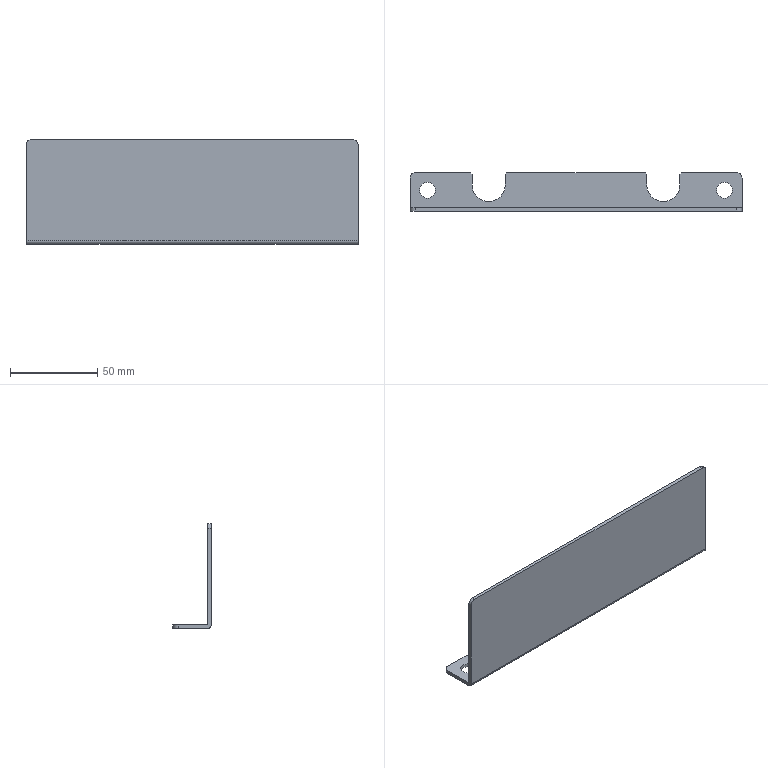Part | STEP file | gslz 2016.10.28-6_id946_x_t | 1 solid | 27 faces | box 190 x 22 x 60 mm | volume 28864 mm3 | plane 18 | cylinder 9 | commonest cylinder face diameters 6 x4 9 x2 19 x2 4 x1
STEP:
#1=CARTESIAN_POINT('',(59.5,282.,2.));
#2=VERTEX_POINT('',#1);
#3=CARTESIAN_POINT('',(59.5,288.,2.));
#4=VERTEX_POINT('',#3);
#5=CARTESIAN_POINT('',(59.5,280.75,2.));
#6=DIRECTION('',(0.,1.,0.));
#7=VECTOR('',#6,1.);
#8=LINE('',#5,#7);
#9=EDGE_CURVE('',#2,#4,#8,.T.);
#10=ORIENTED_EDGE('',*,*,#9,.T.);
#11=CARTESIAN_POINT('',(59.5,288.,0.));
#12=VERTEX_POINT('',#11);
#13=CARTESIAN_POINT('',(59.5,288.,0.));
#14=DIRECTION('',(0.,0.,-1.));
#15=VECTOR('',#14,1.);
#16=LINE('',#13,#15);
#17=EDGE_CURVE('',#4,#12,#16,.T.);
#18=ORIENTED_EDGE('',*,*,#17,.T.);
#19=CARTESIAN_POINT('',(59.5,282.,0.));
#20=VERTEX_POINT('',#19);
#21=CARTESIAN_POINT('',(59.5,280.75,0.));
#22=DIRECTION('',(0.,-1.,0.));
#23=VECTOR('',#22,1.);
#24=LINE('',#21,#23);
#25=EDGE_CURVE('',#12,#20,#24,.T.);
#26=ORIENTED_EDGE('',*,*,#25,.T.);
#27=CARTESIAN_POINT('',(59.5,282.,90.));
#28=DIRECTION('',(0.,0.,-1.));
#29=VECTOR('',#28,1.);
#30=LINE('',#27,#29);
#31=EDGE_CURVE('',#2,#20,#30,.T.);
#32=ORIENTED_EDGE('',*,*,#31,.F.);
#33=EDGE_LOOP('',(#10,#18,#26,#32));
#34=FACE_OUTER_BOUND('',#33,.T.);
#35=CARTESIAN_POINT('',(59.5,280.75,0.));
#36=DIRECTION('',(1.,0.,0.));
#37=DIRECTION('',(0.,0.,1.));
#38=AXIS2_PLACEMENT_3D('',#35,#36,#37);
#39=PLANE('',#38);
#40=ADVANCED_FACE('',(#34),#39,.F.);
#41=CARTESIAN_POINT('',(92.,289.,0.));
#42=VERTEX_POINT('',#41);
#43=CARTESIAN_POINT('',(60.5,289.,0.));
#44=VERTEX_POINT('',#43);
#45=CARTESIAN_POINT('',(0.000000002,289.,0.));
#46=DIRECTION('',(-1.,0.,0.));
#47=VECTOR('',#46,1.);
#48=LINE('',#45,#47);
#49=EDGE_CURVE('',#42,#44,#48,.T.);
#50=ORIENTED_EDGE('',*,*,#49,.T.);
#51=CARTESIAN_POINT('',(60.5,289.,2.));
#52=VERTEX_POINT('',#51);
#53=CARTESIAN_POINT('',(60.5,289.,2.));
#54=DIRECTION('',(0.,0.,1.));
#55=VECTOR('',#54,1.);
#56=LINE('',#53,#55);
#57=EDGE_CURVE('',#44,#52,#56,.T.);
#58=ORIENTED_EDGE('',*,*,#57,.T.);
#59=CARTESIAN_POINT('',(92.,289.,2.));
#60=VERTEX_POINT('',#59);
#61=CARTESIAN_POINT('',(96.45,289.,2.));
#62=DIRECTION('',(-1.,0.,0.));
#63=VECTOR('',#62,1.);
#64=LINE('',#61,#63);
#65=EDGE_CURVE('',#60,#52,#64,.T.);
#66=ORIENTED_EDGE('',*,*,#65,.F.);
#67=CARTESIAN_POINT('',(92.,289.,-221.492));
#68=DIRECTION('',(0.,0.,-1.));
#69=VECTOR('',#68,1.);
#70=LINE('',#67,#69);
#71=EDGE_CURVE('',#60,#42,#70,.T.);
#72=ORIENTED_EDGE('',*,*,#71,.T.);
#73=EDGE_LOOP('',(#50,#58,#66,#72));
#74=FACE_OUTER_BOUND('',#73,.T.);
#75=CARTESIAN_POINT('',(0.000000002,289.,-221.492));
#76=DIRECTION('',(0.,1.,0.));
#77=DIRECTION('',(0.,0.,1.));
#78=AXIS2_PLACEMENT_3D('',#75,#76,#77);
#79=PLANE('',#78);
#80=ADVANCED_FACE('',(#74),#79,.T.);
#81=ORIENTED_EDGE('',*,*,#65,.T.);
#82=CARTESIAN_POINT('',(67.475,295.975,2.));
#83=DIRECTION('',(-0.7071,-0.7071,0.));
#84=VECTOR('',#83,1.);
#85=LINE('',#82,#84);
#86=EDGE_CURVE('',#52,#4,#85,.T.);
#87=ORIENTED_EDGE('',*,*,#86,.T.);
#88=ORIENTED_EDGE('',*,*,#9,.F.);
#89=CARTESIAN_POINT('',(40.5,282.,2.));
#90=VERTEX_POINT('',#89);
#91=CARTESIAN_POINT('',(50.,282.,2.));
#92=DIRECTION('',(0.,0.,1.));
#93=DIRECTION('',(0.,-1.,0.));
#94=AXIS2_PLACEMENT_3D('',#91,#92,#93);
#95=CIRCLE('',#94,9.5);
#96=EDGE_CURVE('',#90,#2,#95,.T.);
#97=ORIENTED_EDGE('',*,*,#96,.F.);
#98=CARTESIAN_POINT('',(40.5,288.,2.));
#99=VERTEX_POINT('',#98);
#100=CARTESIAN_POINT('',(40.5,280.75,2.));
#101=DIRECTION('',(0.,-1.,0.));
#102=VECTOR('',#101,1.);
#103=LINE('',#100,#102);
#104=EDGE_CURVE('',#99,#90,#103,.T.);
#105=ORIENTED_EDGE('',*,*,#104,.F.);
#106=CARTESIAN_POINT('',(39.5,289.,2.));
#107=VERTEX_POINT('',#106);
#108=CARTESIAN_POINT('',(78.975,249.525,2.));
#109=DIRECTION('',(-0.7071,0.7071,0.));
#110=VECTOR('',#109,1.);
#111=LINE('',#108,#110);
#112=EDGE_CURVE('',#99,#107,#111,.T.);
#113=ORIENTED_EDGE('',*,*,#112,.T.);
#114=CARTESIAN_POINT('',(-39.5,289.,2.));
#115=VERTEX_POINT('',#114);
#116=CARTESIAN_POINT('',(96.45,289.,2.));
#117=DIRECTION('',(-1.,0.,0.));
#118=VECTOR('',#117,1.);
#119=LINE('',#116,#118);
#120=EDGE_CURVE('',#107,#115,#119,.T.);
#121=ORIENTED_EDGE('',*,*,#120,.T.);
#122=CARTESIAN_POINT('',(-40.5,288.,2.));
#123=VERTEX_POINT('',#122);
#124=CARTESIAN_POINT('',(17.475,345.975,2.));
#125=DIRECTION('',(-0.7071,-0.7071,0.));
#126=VECTOR('',#125,1.);
#127=LINE('',#124,#126);
#128=EDGE_CURVE('',#115,#123,#127,.T.);
#129=ORIENTED_EDGE('',*,*,#128,.T.);
#130=CARTESIAN_POINT('',(-40.5,282.,2.));
#131=VERTEX_POINT('',#130);
#132=CARTESIAN_POINT('',(-40.5,280.75,2.));
#133=DIRECTION('',(0.,1.,0.));
#134=VECTOR('',#133,1.);
#135=LINE('',#132,#134);
#136=EDGE_CURVE('',#131,#123,#135,.T.);
#137=ORIENTED_EDGE('',*,*,#136,.F.);
#138=CARTESIAN_POINT('',(-59.5,282.,2.));
#139=VERTEX_POINT('',#138);
#140=CARTESIAN_POINT('',(-50.,282.,2.));
#141=DIRECTION('',(0.,0.,1.));
#142=DIRECTION('',(0.,-1.,0.));
#143=AXIS2_PLACEMENT_3D('',#140,#141,#142);
#144=CIRCLE('',#143,9.5);
#145=EDGE_CURVE('',#139,#131,#144,.T.);
#146=ORIENTED_EDGE('',*,*,#145,.F.);
#147=CARTESIAN_POINT('',(-59.5,288.,2.));
#148=VERTEX_POINT('',#147);
#149=CARTESIAN_POINT('',(-59.5,280.75,2.));
#150=DIRECTION('',(0.,-1.,0.));
#151=VECTOR('',#150,1.);
#152=LINE('',#149,#151);
#153=EDGE_CURVE('',#148,#139,#152,.T.);
#154=ORIENTED_EDGE('',*,*,#153,.F.);
#155=CARTESIAN_POINT('',(-60.5,289.,2.));
#156=VERTEX_POINT('',#155);
#157=CARTESIAN_POINT('',(28.975,199.525,2.));
#158=DIRECTION('',(-0.7071,0.7071,0.));
#159=VECTOR('',#158,1.);
#160=LINE('',#157,#159);
#161=EDGE_CURVE('',#148,#156,#160,.T.);
#162=ORIENTED_EDGE('',*,*,#161,.T.);
#163=CARTESIAN_POINT('',(-92.,289.,2.));
#164=VERTEX_POINT('',#163);
#165=CARTESIAN_POINT('',(96.45,289.,2.));
#166=DIRECTION('',(-1.,0.,0.));
#167=VECTOR('',#166,1.);
#168=LINE('',#165,#167);
#169=EDGE_CURVE('',#156,#164,#168,.T.);
#170=ORIENTED_EDGE('',*,*,#169,.T.);
#171=CARTESIAN_POINT('',(-95.,286.,2.));
#172=VERTEX_POINT('',#171);
#173=CARTESIAN_POINT('',(-92.,286.,2.));
#174=DIRECTION('',(0.,0.,1.));
#175=DIRECTION('',(0.,-1.,0.));
#176=AXIS2_PLACEMENT_3D('',#173,#174,#175);
#177=CIRCLE('',#176,3.);
#178=EDGE_CURVE('',#164,#172,#177,.T.);
#179=ORIENTED_EDGE('',*,*,#178,.T.);
#180=CARTESIAN_POINT('',(-95.,269.,2.));
#181=VERTEX_POINT('',#180);
#182=CARTESIAN_POINT('',(-95.,267.,2.));
#183=DIRECTION('',(0.,1.,0.));
#184=VECTOR('',#183,1.);
#185=LINE('',#182,#184);
#186=EDGE_CURVE('',#181,#172,#185,.T.);
#187=ORIENTED_EDGE('',*,*,#186,.F.);
#188=CARTESIAN_POINT('',(95.,269.,2.));
#189=VERTEX_POINT('',#188);
#190=CARTESIAN_POINT('',(-84.45,269.,2.));
#191=DIRECTION('',(-1.,0.,0.));
#192=VECTOR('',#191,1.);
#193=LINE('',#190,#192);
#194=EDGE_CURVE('',#189,#181,#193,.T.);
#195=ORIENTED_EDGE('',*,*,#194,.F.);
#196=CARTESIAN_POINT('',(95.,286.,2.));
#197=VERTEX_POINT('',#196);
#198=CARTESIAN_POINT('',(95.,267.,2.));
#199=DIRECTION('',(0.,-1.,0.));
#200=VECTOR('',#199,1.);
#201=LINE('',#198,#200);
#202=EDGE_CURVE('',#197,#189,#201,.T.);
#203=ORIENTED_EDGE('',*,*,#202,.F.);
#204=CARTESIAN_POINT('',(92.,286.,2.));
#205=DIRECTION('',(0.,0.,1.));
#206=DIRECTION('',(0.,-1.,0.));
#207=AXIS2_PLACEMENT_3D('',#204,#205,#206);
#208=CIRCLE('',#207,3.);
#209=EDGE_CURVE('',#197,#60,#208,.T.);
#210=ORIENTED_EDGE('',*,*,#209,.T.);
#211=EDGE_LOOP('',(#81,#87,#88,#97,#105,#113,#121,#129,#137,#146,#154,#162,#170,#179,#187,#195,#203,#210));
#212=FACE_BOUND('',#211,.T.);
#213=CARTESIAN_POINT('',(-89.5,279.,2.));
#214=VERTEX_POINT('',#213);
#215=CARTESIAN_POINT('',(-85.,279.,2.));
#216=DIRECTION('',(0.,0.,-1.));
#217=DIRECTION('',(-1.,0.,0.));
#218=AXIS2_PLACEMENT_3D('',#215,#216,#217);
#219=CIRCLE('',#218,4.5);
#220=EDGE_CURVE('',#214,#214,#219,.T.);
#221=ORIENTED_EDGE('',*,*,#220,.T.);
#222=EDGE_LOOP('',(#221));
#223=FACE_BOUND('',#222,.T.);
#224=CARTESIAN_POINT('',(80.5,279.,2.));
#225=VERTEX_POINT('',#224);
#226=CARTESIAN_POINT('',(85.,279.,2.));
#227=DIRECTION('',(0.,0.,-1.));
#228=DIRECTION('',(-1.,0.,0.));
#229=AXIS2_PLACEMENT_3D('',#226,#227,#228);
#230=CIRCLE('',#229,4.5);
#231=EDGE_CURVE('',#225,#225,#230,.T.);
#232=ORIENTED_EDGE('',*,*,#231,.T.);
#233=EDGE_LOOP('',(#232));
#234=FACE_BOUND('',#233,.T.);
#235=CARTESIAN_POINT('',(96.45,267.,2.));
#236=DIRECTION('',(0.,0.,1.));
#237=DIRECTION('',(-1.,0.,0.));
#238=AXIS2_PLACEMENT_3D('',#235,#236,#237);
#239=PLANE('',#238);
#240=ADVANCED_FACE('',(#212,#223,#234),#239,.T.);
#241=ORIENTED_EDGE('',*,*,#25,.F.);
#242=CARTESIAN_POINT('',(-41.75,186.75,0.));
#243=DIRECTION('',(0.7071,0.7071,0.));
#244=VECTOR('',#243,1.);
#245=LINE('',#242,#244);
#246=EDGE_CURVE('',#12,#44,#245,.T.);
#247=ORIENTED_EDGE('',*,*,#246,.T.);
#248=ORIENTED_EDGE('',*,*,#49,.F.);
#249=CARTESIAN_POINT('',(95.,286.,0.));
#250=VERTEX_POINT('',#249);
#251=CARTESIAN_POINT('',(92.,286.,0.));
#252=DIRECTION('',(0.,0.,-1.));
#253=DIRECTION('',(0.,-1.,0.));
#254=AXIS2_PLACEMENT_3D('',#251,#252,#253);
#255=CIRCLE('',#254,3.);
#256=EDGE_CURVE('',#42,#250,#255,.T.);
#257=ORIENTED_EDGE('',*,*,#256,.T.);
#258=CARTESIAN_POINT('',(95.,269.,0.));
#259=VERTEX_POINT('',#258);
#260=CARTESIAN_POINT('',(95.,155.,0.));
#261=DIRECTION('',(0.,1.,0.));
#262=VECTOR('',#261,1.);
#263=LINE('',#260,#262);
#264=EDGE_CURVE('',#259,#250,#263,.T.);
#265=ORIENTED_EDGE('',*,*,#264,.F.);
#266=CARTESIAN_POINT('',(-95.,269.,0.));
#267=VERTEX_POINT('',#266);
#268=CARTESIAN_POINT('',(-95.,269.,0.));
#269=DIRECTION('',(-1.,0.,0.));
#270=VECTOR('',#269,1.);
#271=LINE('',#268,#270);
#272=EDGE_CURVE('',#259,#267,#271,.T.);
#273=ORIENTED_EDGE('',*,*,#272,.T.);
#274=CARTESIAN_POINT('',(-95.,286.,0.));
#275=VERTEX_POINT('',#274);
#276=CARTESIAN_POINT('',(-95.,155.,0.));
#277=DIRECTION('',(0.,1.,0.));
#278=VECTOR('',#277,1.);
#279=LINE('',#276,#278);
#280=EDGE_CURVE('',#267,#275,#279,.T.);
#281=ORIENTED_EDGE('',*,*,#280,.T.);
#282=CARTESIAN_POINT('',(-92.,289.,0.));
#283=VERTEX_POINT('',#282);
#284=CARTESIAN_POINT('',(-92.,286.,0.));
#285=DIRECTION('',(0.,0.,-1.));
#286=DIRECTION('',(0.,-1.,0.));
#287=AXIS2_PLACEMENT_3D('',#284,#285,#286);
#288=CIRCLE('',#287,3.);
#289=EDGE_CURVE('',#275,#283,#288,.T.);
#290=ORIENTED_EDGE('',*,*,#289,.T.);
#291=CARTESIAN_POINT('',(-60.5,289.,0.));
#292=VERTEX_POINT('',#291);
#293=CARTESIAN_POINT('',(0.000000002,289.,0.));
#294=DIRECTION('',(-1.,0.,0.));
#295=VECTOR('',#294,1.);
#296=LINE('',#293,#295);
#297=EDGE_CURVE('',#292,#283,#296,.T.);
#298=ORIENTED_EDGE('',*,*,#297,.F.);
#299=CARTESIAN_POINT('',(-59.5,288.,0.));
#300=VERTEX_POINT('',#299);
#301=CARTESIAN_POINT('',(31.75,196.75,0.));
#302=DIRECTION('',(0.7071,-0.7071,0.));
#303=VECTOR('',#302,1.);
#304=LINE('',#301,#303);
#305=EDGE_CURVE('',#292,#300,#304,.T.);
#306=ORIENTED_EDGE('',*,*,#305,.T.);
#307=CARTESIAN_POINT('',(-59.5,282.,0.));
#308=VERTEX_POINT('',#307);
#309=CARTESIAN_POINT('',(-59.5,280.75,0.));
#310=DIRECTION('',(0.,-1.,0.));
#311=VECTOR('',#310,1.);
#312=LINE('',#309,#311);
#313=EDGE_CURVE('',#300,#308,#312,.T.);
#314=ORIENTED_EDGE('',*,*,#313,.T.);
#315=CARTESIAN_POINT('',(-40.5,282.,0.));
#316=VERTEX_POINT('',#315);
#317=CARTESIAN_POINT('',(-50.,282.,0.));
#318=DIRECTION('',(0.,0.,-1.));
#319=DIRECTION('',(-1.,0.,0.));
#320=AXIS2_PLACEMENT_3D('',#317,#318,#319);
#321=CIRCLE('',#320,9.5);
#322=EDGE_CURVE('',#316,#308,#321,.T.);
#323=ORIENTED_EDGE('',*,*,#322,.F.);
#324=CARTESIAN_POINT('',(-40.5,288.,0.));
#325=VERTEX_POINT('',#324);
#326=CARTESIAN_POINT('',(-40.5,280.75,0.));
#327=DIRECTION('',(0.,1.,0.));
#328=VECTOR('',#327,1.);
#329=LINE('',#326,#328);
#330=EDGE_CURVE('',#316,#325,#329,.T.);
#331=ORIENTED_EDGE('',*,*,#330,.T.);
#332=CARTESIAN_POINT('',(-39.5,289.,0.));
#333=VERTEX_POINT('',#332);
#334=CARTESIAN_POINT('',(-91.75,236.75,0.));
#335=DIRECTION('',(0.7071,0.7071,0.));
#336=VECTOR('',#335,1.);
#337=LINE('',#334,#336);
#338=EDGE_CURVE('',#325,#333,#337,.T.);
#339=ORIENTED_EDGE('',*,*,#338,.T.);
#340=CARTESIAN_POINT('',(39.5,289.,0.));
#341=VERTEX_POINT('',#340);
#342=CARTESIAN_POINT('',(0.000000002,289.,0.));
#343=DIRECTION('',(-1.,0.,0.));
#344=VECTOR('',#343,1.);
#345=LINE('',#342,#344);
#346=EDGE_CURVE('',#341,#333,#345,.T.);
#347=ORIENTED_EDGE('',*,*,#346,.F.);
#348=CARTESIAN_POINT('',(40.5,288.,0.));
#349=VERTEX_POINT('',#348);
#350=CARTESIAN_POINT('',(81.75,246.75,0.));
#351=DIRECTION('',(0.7071,-0.7071,0.));
#352=VECTOR('',#351,1.);
#353=LINE('',#350,#352);
#354=EDGE_CURVE('',#341,#349,#353,.T.);
#355=ORIENTED_EDGE('',*,*,#354,.T.);
#356=CARTESIAN_POINT('',(40.5,282.,0.));
#357=VERTEX_POINT('',#356);
#358=CARTESIAN_POINT('',(40.5,280.75,0.));
#359=DIRECTION('',(0.,-1.,0.));
#360=VECTOR('',#359,1.);
#361=LINE('',#358,#360);
#362=EDGE_CURVE('',#349,#357,#361,.T.);
#363=ORIENTED_EDGE('',*,*,#362,.T.);
#364=CARTESIAN_POINT('',(50.,282.,0.));
#365=DIRECTION('',(0.,0.,-1.));
#366=DIRECTION('',(-1.,0.,0.));
#367=AXIS2_PLACEMENT_3D('',#364,#365,#366);
#368=CIRCLE('',#367,9.5);
#369=EDGE_CURVE('',#20,#357,#368,.T.);
#370=ORIENTED_EDGE('',*,*,#369,.F.);
#371=EDGE_LOOP('',(#241,#247,#248,#257,#265,#273,#281,#290,#298,#306,#314,#323,#331,#339,#347,#355,#363,#370));
#372=FACE_BOUND('',#371,.T.);
#373=CARTESIAN_POINT('',(80.5,279.,0.));
#374=VERTEX_POINT('',#373);
#375=CARTESIAN_POINT('',(85.,279.,0.));
#376=DIRECTION('',(0.,0.,-1.));
#377=DIRECTION('',(-1.,0.,0.));
#378=AXIS2_PLACEMENT_3D('',#375,#376,#377);
#379=CIRCLE('',#378,4.5);
#380=EDGE_CURVE('',#374,#374,#379,.T.);
#381=ORIENTED_EDGE('',*,*,#380,.F.);
#382=EDGE_LOOP('',(#381));
#383=FACE_BOUND('',#382,.T.);
#384=CARTESIAN_POINT('',(-89.5,279.,0.));
#385=VERTEX_POINT('',#384);
#386=CARTESIAN_POINT('',(-85.,279.,0.));
#387=DIRECTION('',(0.,0.,-1.));
#388=DIRECTION('',(-1.,0.,0.));
#389=AXIS2_PLACEMENT_3D('',#386,#387,#388);
#390=CIRCLE('',#389,4.5);
#391=EDGE_CURVE('',#385,#385,#390,.T.);
#392=ORIENTED_EDGE('',*,*,#391,.F.);
#393=EDGE_LOOP('',(#392));
#394=FACE_BOUND('',#393,.T.);
#395=CARTESIAN_POINT('',(-10.,155.,0.));
#396=DIRECTION('',(0.,0.,1.));
#397=DIRECTION('',(-1.,0.,0.));
#398=AXIS2_PLACEMENT_3D('',#395,#396,#397);
#399=PLANE('',#398);
#400=ADVANCED_FACE('',(#372,#383,#394),#399,.F.);
#401=ORIENTED_EDGE('',*,*,#120,.F.);
#402=CARTESIAN_POINT('',(39.5,289.,0.));
#403=DIRECTION('',(0.,0.,-1.));
#404=VECTOR('',#403,1.);
#405=LINE('',#402,#404);
#406=EDGE_CURVE('',#107,#341,#405,.T.);
#407=ORIENTED_EDGE('',*,*,#406,.T.);
#408=ORIENTED_EDGE('',*,*,#346,.T.);
#409=CARTESIAN_POINT('',(-39.5,289.,2.));
#410=DIRECTION('',(0.,0.,1.));
#411=VECTOR('',#410,1.);
#412=LINE('',#409,#411);
#413=EDGE_CURVE('',#333,#115,#412,.T.);
#414=ORIENTED_EDGE('',*,*,#413,.T.);
#415=EDGE_LOOP('',(#401,#407,#408,#414));
#416=FACE_OUTER_BOUND('',#415,.T.);
#417=CARTESIAN_POINT('',(0.000000002,289.,-221.492));
#418=DIRECTION('',(0.,1.,0.));
#419=DIRECTION('',(0.,0.,1.));
#420=AXIS2_PLACEMENT_3D('',#417,#418,#419);
#421=PLANE('',#420);
#422=ADVANCED_FACE('',(#416),#421,.T.);
#423=ORIENTED_EDGE('',*,*,#186,.T.);
#424=CARTESIAN_POINT('',(-95.,286.,0.));
#425=DIRECTION('',(0.,0.,-1.));
#426=VECTOR('',#425,1.);
#427=LINE('',#424,#426);
#428=EDGE_CURVE('',#172,#275,#427,.T.);
#429=ORIENTED_EDGE('',*,*,#428,.T.);
#430=ORIENTED_EDGE('',*,*,#280,.F.);
#431=CARTESIAN_POINT('',(-95.,267.,2.));
#432=VERTEX_POINT('',#431);
#433=CARTESIAN_POINT('',(-95.,269.,2.));
#434=DIRECTION('',(-1.,0.,0.));
#435=DIRECTION('',(0.,0.,1.));
#436=AXIS2_PLACEMENT_3D('',#433,#434,#435);
#437=CIRCLE('',#436,2.);
#438=EDGE_CURVE('',#267,#432,#437,.T.);
#439=ORIENTED_EDGE('',*,*,#438,.T.);
#440=CARTESIAN_POINT('',(-95.,267.,57.));
#441=VERTEX_POINT('',#440);
#442=CARTESIAN_POINT('',(-95.,267.,2.));
#443=DIRECTION('',(0.,0.,-1.));
#444=VECTOR('',#443,1.);
#445=LINE('',#442,#444);
#446=EDGE_CURVE('',#441,#432,#445,.T.);
#447=ORIENTED_EDGE('',*,*,#446,.F.);
#448=CARTESIAN_POINT('',(-95.,269.,57.));
#449=VERTEX_POINT('',#448);
#450=CARTESIAN_POINT('',(-95.,0.,57.));
#451=DIRECTION('',(0.,1.,0.));
#452=VECTOR('',#451,1.);
#453=LINE('',#450,#452);
#454=EDGE_CURVE('',#441,#449,#453,.T.);
#455=ORIENTED_EDGE('',*,*,#454,.T.);
#456=CARTESIAN_POINT('',(-95.,269.,2.));
#457=DIRECTION('',(0.,0.,-1.));
#458=VECTOR('',#457,1.);
#459=LINE('',#456,#458);
#460=EDGE_CURVE('',#449,#181,#459,.T.);
#461=ORIENTED_EDGE('',*,*,#460,.T.);
#462=EDGE_LOOP('',(#423,#429,#430,#439,#447,#455,#461));
#463=FACE_OUTER_BOUND('',#462,.T.);
#464=CARTESIAN_POINT('',(-95.,0.,0.));
#465=DIRECTION('',(-1.,0.,0.));
#466=DIRECTION('',(0.,0.,-1.));
#467=AXIS2_PLACEMENT_3D('',#464,#465,#466);
#468=PLANE('',#467);
#469=ADVANCED_FACE('',(#463),#468,.T.);
#470=ORIENTED_EDGE('',*,*,#264,.T.);
#471=CARTESIAN_POINT('',(95.,286.,0.));
#472=DIRECTION('',(0.,0.,1.));
#473=VECTOR('',#472,1.);
#474=LINE('',#471,#473);
#475=EDGE_CURVE('',#250,#197,#474,.T.);
#476=ORIENTED_EDGE('',*,*,#475,.T.);
#477=ORIENTED_EDGE('',*,*,#202,.T.);
#478=CARTESIAN_POINT('',(95.,269.,57.));
#479=VERTEX_POINT('',#478);
#480=CARTESIAN_POINT('',(95.,269.,2.));
#481=DIRECTION('',(0.,0.,1.));
#482=VECTOR('',#481,1.);
#483=LINE('',#480,#482);
#484=EDGE_CURVE('',#189,#479,#483,.T.);
#485=ORIENTED_EDGE('',*,*,#484,.T.);
#486=CARTESIAN_POINT('',(95.,267.,57.));
#487=VERTEX_POINT('',#486);
#488=CARTESIAN_POINT('',(95.,0.,57.));
#489=DIRECTION('',(0.,-1.,0.));
#490=VECTOR('',#489,1.);
#491=LINE('',#488,#490);
#492=EDGE_CURVE('',#479,#487,#491,.T.);
#493=ORIENTED_EDGE('',*,*,#492,.T.);
#494=CARTESIAN_POINT('',(95.,267.,2.));
#495=VERTEX_POINT('',#494);
#496=CARTESIAN_POINT('',(95.,267.,2.));
#497=DIRECTION('',(0.,0.,1.));
#498=VECTOR('',#497,1.);
#499=LINE('',#496,#498);
#500=EDGE_CURVE('',#495,#487,#499,.T.);
#501=ORIENTED_EDGE('',*,*,#500,.F.);
#502=CARTESIAN_POINT('',(95.,269.,2.));
#503=DIRECTION('',(1.,0.,0.));
#504=DIRECTION('',(0.,0.,-1.));
#505=AXIS2_PLACEMENT_3D('',#502,#503,#504);
#506=CIRCLE('',#505,2.);
#507=EDGE_CURVE('',#495,#259,#506,.T.);
#508=ORIENTED_EDGE('',*,*,#507,.T.);
#509=EDGE_LOOP('',(#470,#476,#477,#485,#493,#501,#508));
#510=FACE_OUTER_BOUND('',#509,.T.);
#511=CARTESIAN_POINT('',(95.,0.,0.));
#512=DIRECTION('',(1.,0.,0.));
#513=DIRECTION('',(0.,0.,1.));
#514=AXIS2_PLACEMENT_3D('',#511,#512,#513);
#515=PLANE('',#514);
#516=ADVANCED_FACE('',(#510),#515,.T.);
#517=CARTESIAN_POINT('',(-92.,269.,60.));
#518=VERTEX_POINT('',#517);
#519=CARTESIAN_POINT('',(92.,269.,60.));
#520=VERTEX_POINT('',#519);
#521=CARTESIAN_POINT('',(-89.5,269.,60.));
#522=DIRECTION('',(1.,0.,0.));
#523=VECTOR('',#522,1.);
#524=LINE('',#521,#523);
#525=EDGE_CURVE('',#518,#520,#524,.T.);
#526=ORIENTED_EDGE('',*,*,#525,.F.);
#527=CARTESIAN_POINT('',(-92.,267.,60.));
#528=VERTEX_POINT('',#527);
#529=CARTESIAN_POINT('',(-92.,200.,60.));
#530=DIRECTION('',(0.,-1.,0.));
#531=VECTOR('',#530,1.);
#532=LINE('',#529,#531);
#533=EDGE_CURVE('',#518,#528,#532,.T.);
#534=ORIENTED_EDGE('',*,*,#533,.T.);
#535=CARTESIAN_POINT('',(92.,267.,60.));
#536=VERTEX_POINT('',#535);
#537=CARTESIAN_POINT('',(-89.5,267.,60.));
#538=DIRECTION('',(1.,0.,0.));
#539=VECTOR('',#538,1.);
#540=LINE('',#537,#539);
#541=EDGE_CURVE('',#528,#536,#540,.T.);
#542=ORIENTED_EDGE('',*,*,#541,.T.);
#543=CARTESIAN_POINT('',(92.,200.,60.));
#544=DIRECTION('',(0.,1.,0.));
#545=VECTOR('',#544,1.);
#546=LINE('',#543,#545);
#547=EDGE_CURVE('',#536,#520,#546,.T.);
#548=ORIENTED_EDGE('',*,*,#547,.T.);
#549=EDGE_LOOP('',(#526,#534,#542,#548));
#550=FACE_OUTER_BOUND('',#549,.T.);
#551=CARTESIAN_POINT('',(-89.5,200.,60.));
#552=DIRECTION('',(0.,0.,1.));
#553=DIRECTION('',(-1.,0.,0.));
#554=AXIS2_PLACEMENT_3D('',#551,#552,#553);
#555=PLANE('',#554);
#556=ADVANCED_FACE('',(#550),#555,.T.);
#557=ORIENTED_EDGE('',*,*,#169,.F.);
#558=CARTESIAN_POINT('',(-60.5,289.,0.));
#559=DIRECTION('',(0.,0.,-1.));
#560=VECTOR('',#559,1.);
#561=LINE('',#558,#560);
#562=EDGE_CURVE('',#156,#292,#561,.T.);
#563=ORIENTED_EDGE('',*,*,#562,.T.);
#564=ORIENTED_EDGE('',*,*,#297,.T.);
#565=CARTESIAN_POINT('',(-92.,289.,-221.492));
#566=DIRECTION('',(0.,0.,1.));
#567=VECTOR('',#566,1.);
#568=LINE('',#565,#567);
#569=EDGE_CURVE('',#283,#164,#568,.T.);
#570=ORIENTED_EDGE('',*,*,#569,.T.);
#571=EDGE_LOOP('',(#557,#563,#564,#570));
#572=FACE_OUTER_BOUND('',#571,.T.);
#573=CARTESIAN_POINT('',(0.000000002,289.,-221.492));
#574=DIRECTION('',(0.,1.,0.));
#575=DIRECTION('',(0.,0.,1.));
#576=AXIS2_PLACEMENT_3D('',#573,#574,#575);
#577=PLANE('',#576);
#578=ADVANCED_FACE('',(#572),#577,.T.);
#579=ORIENTED_EDGE('',*,*,#541,.F.);
#580=CARTESIAN_POINT('',(-92.,267.,57.));
#581=DIRECTION('',(0.,-1.,0.));
#582=DIRECTION('',(-1.,0.,0.));
#583=AXIS2_PLACEMENT_3D('',#580,#581,#582);
#584=CIRCLE('',#583,3.);
#585=EDGE_CURVE('',#528,#441,#584,.T.);
#586=ORIENTED_EDGE('',*,*,#585,.T.);
#587=ORIENTED_EDGE('',*,*,#446,.T.);
#588=CARTESIAN_POINT('',(95.,267.,2.));
#589=DIRECTION('',(1.,0.,0.));
#590=VECTOR('',#589,1.);
#591=LINE('',#588,#590);
#592=EDGE_CURVE('',#432,#495,#591,.T.);
#593=ORIENTED_EDGE('',*,*,#592,.T.);
#594=ORIENTED_EDGE('',*,*,#500,.T.);
#595=CARTESIAN_POINT('',(92.,267.,57.));
#596=DIRECTION('',(0.,-1.,0.));
#597=DIRECTION('',(-1.,0.,0.));
#598=AXIS2_PLACEMENT_3D('',#595,#596,#597);
#599=CIRCLE('',#598,3.);
#600=EDGE_CURVE('',#487,#536,#599,.T.);
#601=ORIENTED_EDGE('',*,*,#600,.T.);
#602=EDGE_LOOP('',(#579,#586,#587,#593,#594,#601));
#603=FACE_OUTER_BOUND('',#602,.T.);
#604=CARTESIAN_POINT('',(-89.45,267.,2.));
#605=DIRECTION('',(0.,1.,0.));
#606=DIRECTION('',(0.,0.,1.));
#607=AXIS2_PLACEMENT_3D('',#604,#605,#606);
#608=PLANE('',#607);
#609=ADVANCED_FACE('',(#603),#608,.F.);
#610=ORIENTED_EDGE('',*,*,#460,.F.);
#611=CARTESIAN_POINT('',(-92.,269.,57.));
#612=DIRECTION('',(0.,1.,0.));
#613=DIRECTION('',(-1.,0.,0.));
#614=AXIS2_PLACEMENT_3D('',#611,#612,#613);
#615=CIRCLE('',#614,3.);
#616=EDGE_CURVE('',#449,#518,#615,.T.);
#617=ORIENTED_EDGE('',*,*,#616,.T.);
#618=ORIENTED_EDGE('',*,*,#525,.T.);
#619=CARTESIAN_POINT('',(92.,269.,57.));
#620=DIRECTION('',(0.,1.,0.));
#621=DIRECTION('',(-1.,0.,0.));
#622=AXIS2_PLACEMENT_3D('',#619,#620,#621);
#623=CIRCLE('',#622,3.);
#624=EDGE_CURVE('',#520,#479,#623,.T.);
#625=ORIENTED_EDGE('',*,*,#624,.T.);
#626=ORIENTED_EDGE('',*,*,#484,.F.);
#627=ORIENTED_EDGE('',*,*,#194,.T.);
#628=EDGE_LOOP('',(#610,#617,#618,#625,#626,#627));
#629=FACE_OUTER_BOUND('',#628,.T.);
#630=CARTESIAN_POINT('',(-89.45,269.,2.));
#631=DIRECTION('',(0.,1.,0.));
#632=DIRECTION('',(0.,0.,1.));
#633=AXIS2_PLACEMENT_3D('',#630,#631,#632);
#634=PLANE('',#633);
#635=ADVANCED_FACE('',(#629),#634,.T.);
#636=ORIENTED_EDGE('',*,*,#438,.F.);
#637=ORIENTED_EDGE('',*,*,#272,.F.);
#638=ORIENTED_EDGE('',*,*,#507,.F.);
#639=ORIENTED_EDGE('',*,*,#592,.F.);
#640=EDGE_LOOP('',(#636,#637,#638,#639));
#641=FACE_OUTER_BOUND('',#640,.T.);
#642=CARTESIAN_POINT('',(-89.45,269.,2.));
#643=DIRECTION('',(1.,0.,0.));
#644=DIRECTION('',(0.,1.,0.));
#645=AXIS2_PLACEMENT_3D('',#642,#643,#644);
#646=CYLINDRICAL_SURFACE('',#645,2.);
#647=ADVANCED_FACE('',(#641),#646,.T.);
#648=ORIENTED_EDGE('',*,*,#391,.T.);
#649=EDGE_LOOP('',(#648));
#650=FACE_BOUND('',#649,.T.);
#651=ORIENTED_EDGE('',*,*,#220,.F.);
#652=EDGE_LOOP('',(#651));
#653=FACE_BOUND('',#652,.T.);
#654=CARTESIAN_POINT('',(-85.,279.,0.));
#655=DIRECTION('',(0.,0.,-1.));
#656=DIRECTION('',(-1.,0.,0.));
#657=AXIS2_PLACEMENT_3D('',#654,#655,#656);
#658=CYLINDRICAL_SURFACE('',#657,4.5);
#659=ADVANCED_FACE('',(#650,#653),#658,.F.);
#660=ORIENTED_EDGE('',*,*,#380,.T.);
#661=EDGE_LOOP('',(#660));
#662=FACE_BOUND('',#661,.T.);
#663=ORIENTED_EDGE('',*,*,#231,.F.);
#664=EDGE_LOOP('',(#663));
#665=FACE_BOUND('',#664,.T.);
#666=CARTESIAN_POINT('',(85.,279.,0.));
#667=DIRECTION('',(0.,0.,-1.));
#668=DIRECTION('',(1.,0.,0.));
#669=AXIS2_PLACEMENT_3D('',#666,#667,#668);
#670=CYLINDRICAL_SURFACE('',#669,4.5);
#671=ADVANCED_FACE('',(#662,#665),#670,.F.);
#672=ORIENTED_EDGE('',*,*,#289,.F.);
#673=ORIENTED_EDGE('',*,*,#428,.F.);
#674=ORIENTED_EDGE('',*,*,#178,.F.);
#675=ORIENTED_EDGE('',*,*,#569,.F.);
#676=EDGE_LOOP('',(#672,#673,#674,#675));
#677=FACE_OUTER_BOUND('',#676,.T.);
#678=CARTESIAN_POINT('',(-92.,286.,-221.492));
#679=DIRECTION('',(0.,0.,1.));
#680=DIRECTION('',(0.,1.,0.));
#681=AXIS2_PLACEMENT_3D('',#678,#679,#680);
#682=CYLINDRICAL_SURFACE('',#681,3.);
#683=ADVANCED_FACE('',(#677),#682,.T.);
#684=ORIENTED_EDGE('',*,*,#585,.F.);
#685=ORIENTED_EDGE('',*,*,#533,.F.);
#686=ORIENTED_EDGE('',*,*,#616,.F.);
#687=ORIENTED_EDGE('',*,*,#454,.F.);
#688=EDGE_LOOP('',(#684,#685,#686,#687));
#689=FACE_OUTER_BOUND('',#688,.T.);
#690=CARTESIAN_POINT('',(-92.,0.,57.));
#691=DIRECTION('',(0.,1.,0.));
#692=DIRECTION('',(0.,0.,1.));
#693=AXIS2_PLACEMENT_3D('',#690,#691,#692);
#694=CYLINDRICAL_SURFACE('',#693,3.);
#695=ADVANCED_FACE('',(#689),#694,.T.);
#696=ORIENTED_EDGE('',*,*,#209,.F.);
#697=ORIENTED_EDGE('',*,*,#475,.F.);
#698=ORIENTED_EDGE('',*,*,#256,.F.);
#699=ORIENTED_EDGE('',*,*,#71,.F.);
#700=EDGE_LOOP('',(#696,#697,#698,#699));
#701=FACE_OUTER_BOUND('',#700,.T.);
#702=CARTESIAN_POINT('',(92.,286.,-221.492));
#703=DIRECTION('',(0.,0.,-1.));
#704=DIRECTION('',(0.,1.,0.));
#705=AXIS2_PLACEMENT_3D('',#702,#703,#704);
#706=CYLINDRICAL_SURFACE('',#705,3.);
#707=ADVANCED_FACE('',(#701),#706,.T.);
#708=ORIENTED_EDGE('',*,*,#600,.F.);
#709=ORIENTED_EDGE('',*,*,#492,.F.);
#710=ORIENTED_EDGE('',*,*,#624,.F.);
#711=ORIENTED_EDGE('',*,*,#547,.F.);
#712=EDGE_LOOP('',(#708,#709,#710,#711));
#713=FACE_OUTER_BOUND('',#712,.T.);
#714=CARTESIAN_POINT('',(92.,200.,57.));
#715=DIRECTION('',(0.,1.,0.));
#716=DIRECTION('',(0.,0.,1.));
#717=AXIS2_PLACEMENT_3D('',#714,#715,#716);
#718=CYLINDRICAL_SURFACE('',#717,3.);
#719=ADVANCED_FACE('',(#713),#718,.T.);
#720=ORIENTED_EDGE('',*,*,#136,.T.);
#721=CARTESIAN_POINT('',(-40.5,288.,0.));
#722=DIRECTION('',(0.,0.,-1.));
#723=VECTOR('',#722,1.);
#724=LINE('',#721,#723);
#725=EDGE_CURVE('',#123,#325,#724,.T.);
#726=ORIENTED_EDGE('',*,*,#725,.T.);
#727=ORIENTED_EDGE('',*,*,#330,.F.);
#728=CARTESIAN_POINT('',(-40.5,282.,90.));
#729=DIRECTION('',(0.,0.,1.));
#730=VECTOR('',#729,1.);
#731=LINE('',#728,#730);
#732=EDGE_CURVE('',#316,#131,#731,.T.);
#733=ORIENTED_EDGE('',*,*,#732,.T.);
#734=EDGE_LOOP('',(#720,#726,#727,#733));
#735=FACE_OUTER_BOUND('',#734,.T.);
#736=CARTESIAN_POINT('',(-40.5,280.75,0.));
#737=DIRECTION('',(1.,0.,0.));
#738=DIRECTION('',(0.,0.,-1.));
#739=AXIS2_PLACEMENT_3D('',#736,#737,#738);
#740=PLANE('',#739);
#741=ADVANCED_FACE('',(#735),#740,.F.);
#742=ORIENTED_EDGE('',*,*,#313,.F.);
#743=CARTESIAN_POINT('',(-59.5,288.,2.));
#744=DIRECTION('',(0.,0.,1.));
#745=VECTOR('',#744,1.);
#746=LINE('',#743,#745);
#747=EDGE_CURVE('',#300,#148,#746,.T.);
#748=ORIENTED_EDGE('',*,*,#747,.T.);
#749=ORIENTED_EDGE('',*,*,#153,.T.);
#750=CARTESIAN_POINT('',(-59.5,282.,90.));
#751=DIRECTION('',(0.,0.,-1.));
#752=VECTOR('',#751,1.);
#753=LINE('',#750,#752);
#754=EDGE_CURVE('',#139,#308,#753,.T.);
#755=ORIENTED_EDGE('',*,*,#754,.T.);
#756=EDGE_LOOP('',(#742,#748,#749,#755));
#757=FACE_OUTER_BOUND('',#756,.T.);
#758=CARTESIAN_POINT('',(-59.5,280.75,0.));
#759=DIRECTION('',(-1.,0.,0.));
#760=DIRECTION('',(0.,0.,-1.));
#761=AXIS2_PLACEMENT_3D('',#758,#759,#760);
#762=PLANE('',#761);
#763=ADVANCED_FACE('',(#757),#762,.F.);
#764=ORIENTED_EDGE('',*,*,#362,.F.);
#765=CARTESIAN_POINT('',(40.5,288.,2.));
#766=DIRECTION('',(0.,0.,1.));
#767=VECTOR('',#766,1.);
#768=LINE('',#765,#767);
#769=EDGE_CURVE('',#349,#99,#768,.T.);
#770=ORIENTED_EDGE('',*,*,#769,.T.);
#771=ORIENTED_EDGE('',*,*,#104,.T.);
#772=CARTESIAN_POINT('',(40.5,282.,90.));
#773=DIRECTION('',(0.,0.,-1.));
#774=VECTOR('',#773,1.);
#775=LINE('',#772,#774);
#776=EDGE_CURVE('',#90,#357,#775,.T.);
#777=ORIENTED_EDGE('',*,*,#776,.T.);
#778=EDGE_LOOP('',(#764,#770,#771,#777));
#779=FACE_OUTER_BOUND('',#778,.T.);
#780=CARTESIAN_POINT('',(40.5,280.75,0.));
#781=DIRECTION('',(-1.,0.,0.));
#782=DIRECTION('',(0.,0.,-1.));
#783=AXIS2_PLACEMENT_3D('',#780,#781,#782);
#784=PLANE('',#783);
#785=ADVANCED_FACE('',(#779),#784,.F.);
#786=ORIENTED_EDGE('',*,*,#96,.T.);
#787=ORIENTED_EDGE('',*,*,#31,.T.);
#788=ORIENTED_EDGE('',*,*,#369,.T.);
#789=ORIENTED_EDGE('',*,*,#776,.F.);
#790=EDGE_LOOP('',(#786,#787,#788,#789));
#791=FACE_OUTER_BOUND('',#790,.T.);
#792=CARTESIAN_POINT('',(50.,282.,90.));
#793=DIRECTION('',(0.,0.,-1.));
#794=DIRECTION('',(-1.,0.,0.));
#795=AXIS2_PLACEMENT_3D('',#792,#793,#794);
#796=CYLINDRICAL_SURFACE('',#795,9.5);
#797=ADVANCED_FACE('',(#791),#796,.F.);
#798=ORIENTED_EDGE('',*,*,#145,.T.);
#799=ORIENTED_EDGE('',*,*,#732,.F.);
#800=ORIENTED_EDGE('',*,*,#322,.T.);
#801=ORIENTED_EDGE('',*,*,#754,.F.);
#802=EDGE_LOOP('',(#798,#799,#800,#801));
#803=FACE_OUTER_BOUND('',#802,.T.);
#804=CARTESIAN_POINT('',(-50.,282.,90.));
#805=DIRECTION('',(0.,0.,-1.));
#806=DIRECTION('',(-1.,0.,0.));
#807=AXIS2_PLACEMENT_3D('',#804,#805,#806);
#808=CYLINDRICAL_SURFACE('',#807,9.5);
#809=ADVANCED_FACE('',(#803),#808,.F.);
#810=ORIENTED_EDGE('',*,*,#86,.F.);
#811=ORIENTED_EDGE('',*,*,#57,.F.);
#812=ORIENTED_EDGE('',*,*,#246,.F.);
#813=ORIENTED_EDGE('',*,*,#17,.F.);
#814=EDGE_LOOP('',(#810,#811,#812,#813));
#815=FACE_OUTER_BOUND('',#814,.T.);
#816=CARTESIAN_POINT('',(59.5,288.,0.));
#817=DIRECTION('',(-0.7071,0.7071,0.));
#818=DIRECTION('',(-0.7071,-0.7071,0.));
#819=AXIS2_PLACEMENT_3D('',#816,#817,#818);
#820=PLANE('',#819);
#821=ADVANCED_FACE('',(#815),#820,.T.);
#822=ORIENTED_EDGE('',*,*,#354,.F.);
#823=ORIENTED_EDGE('',*,*,#406,.F.);
#824=ORIENTED_EDGE('',*,*,#112,.F.);
#825=ORIENTED_EDGE('',*,*,#769,.F.);
#826=EDGE_LOOP('',(#822,#823,#824,#825));
#827=FACE_OUTER_BOUND('',#826,.T.);
#828=CARTESIAN_POINT('',(40.5,288.,0.));
#829=DIRECTION('',(0.7071,0.7071,0.));
#830=DIRECTION('',(-0.7071,0.7071,0.));
#831=AXIS2_PLACEMENT_3D('',#828,#829,#830);
#832=PLANE('',#831);
#833=ADVANCED_FACE('',(#827),#832,.T.);
#834=ORIENTED_EDGE('',*,*,#338,.F.);
#835=ORIENTED_EDGE('',*,*,#725,.F.);
#836=ORIENTED_EDGE('',*,*,#128,.F.);
#837=ORIENTED_EDGE('',*,*,#413,.F.);
#838=EDGE_LOOP('',(#834,#835,#836,#837));
#839=FACE_OUTER_BOUND('',#838,.T.);
#840=CARTESIAN_POINT('',(-39.5,289.,-221.492));
#841=DIRECTION('',(-0.7071,0.7071,0.));
#842=DIRECTION('',(-0.7071,-0.7071,0.));
#843=AXIS2_PLACEMENT_3D('',#840,#841,#842);
#844=PLANE('',#843);
#845=ADVANCED_FACE('',(#839),#844,.T.);
#846=ORIENTED_EDGE('',*,*,#305,.F.);
#847=ORIENTED_EDGE('',*,*,#562,.F.);
#848=ORIENTED_EDGE('',*,*,#161,.F.);
#849=ORIENTED_EDGE('',*,*,#747,.F.);
#850=EDGE_LOOP('',(#846,#847,#848,#849));
#851=FACE_OUTER_BOUND('',#850,.T.);
#852=CARTESIAN_POINT('',(-59.5,288.,0.));
#853=DIRECTION('',(0.7071,0.7071,0.));
#854=DIRECTION('',(-0.7071,0.7071,0.));
#855=AXIS2_PLACEMENT_3D('',#852,#853,#854);
#856=PLANE('',#855);
#857=ADVANCED_FACE('',(#851),#856,.T.);
#858=CLOSED_SHELL('',(#40,#80,#240,#400,#422,#469,#516,#556,#578,#609,#635,#647,#659,#671,#683,#695,#707,#719,#741,#763,#785,#797,#809,#821,#833,#845,#857));
#859=MANIFOLD_SOLID_BREP('',#858);
#860=(LENGTH_UNIT()NAMED_UNIT(*)SI_UNIT(.MILLI.,.METRE.));
#861=UNCERTAINTY_MEASURE_WITH_UNIT(LENGTH_MEASURE(0.00002),#860,'','');
#862=(NAMED_UNIT(*)PLANE_ANGLE_UNIT()SI_UNIT($,.RADIAN.));
#863=PLANE_ANGLE_MEASURE_WITH_UNIT(PLANE_ANGLE_MEASURE(0.01745),#862);
#864=DIMENSIONAL_EXPONENTS(0.,0.,0.,0.,0.,0.,0.);
#865=(CONVERSION_BASED_UNIT('DEGREE',#863)NAMED_UNIT(#864)PLANE_ANGLE_UNIT());
#866=(NAMED_UNIT(*)SI_UNIT($,.STERADIAN.)SOLID_ANGLE_UNIT());
#867=(GEOMETRIC_REPRESENTATION_CONTEXT(3)GLOBAL_UNCERTAINTY_ASSIGNED_CONTEXT((#861))GLOBAL_UNIT_ASSIGNED_CONTEXT((#860,#865,#866))REPRESENTATION_CONTEXT('',''));
#868=ADVANCED_BREP_SHAPE_REPRESENTATION('',(#859),#867);